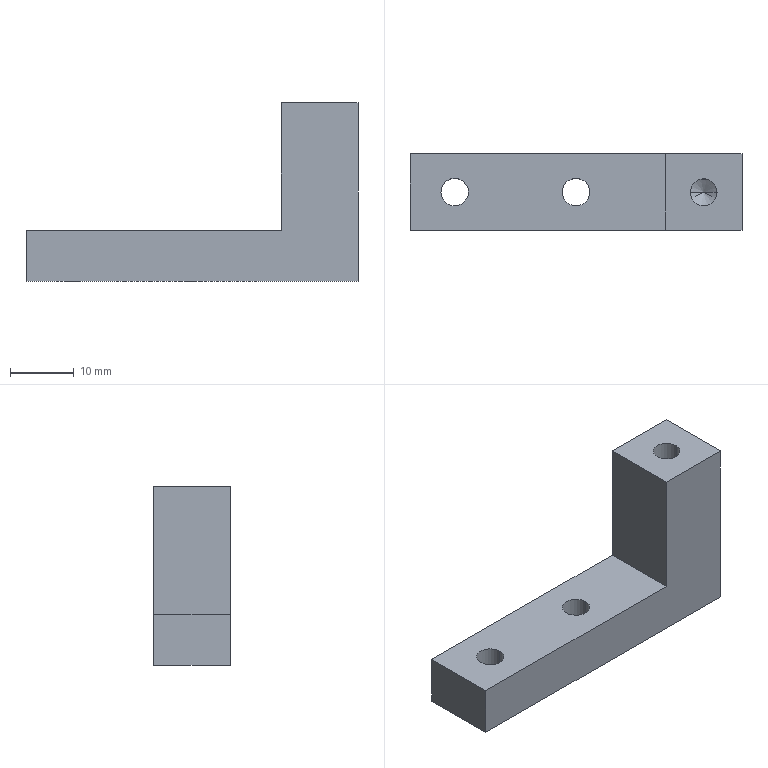Part | STEP file | PN_0008 | 1 solid | 16 faces | box 52 x 12 x 28 mm | volume 7462 mm3 | plane 8 | cylinder 6 | cone 2 | commonest cylinder face diameters 4.3 x4 4.2 x2
STEP:
#1=CARTESIAN_POINT('',(0.,0.,0.));
#2=DIRECTION('',(0.,0.,1.));
#3=DIRECTION('',(1.,0.,0.));
#4=AXIS2_PLACEMENT_3D('',#1,#2,#3);
#5=CARTESIAN_POINT('',(-35.15,6.,0.));
#6=VERTEX_POINT('',#5);
#7=CARTESIAN_POINT('',(-35.15,6.,-8.));
#8=VERTEX_POINT('',#7);
#9=CARTESIAN_POINT('',(-35.15,6.,-8.));
#10=DIRECTION('',(0.,0.,-1.));
#11=VECTOR('',#10,1.);
#12=LINE('',#9,#11);
#13=CARTESIAN_POINT('',(-33.,6.,-8.));
#14=DIRECTION('',(0.,0.,-1.));
#15=DIRECTION('',(-1.,0.,0.));
#16=AXIS2_PLACEMENT_3D('',#13,#14,#15);
#17=CYLINDRICAL_SURFACE('',#16,2.15);
#18=CARTESIAN_POINT('',(6.283,0.));
#19=DIRECTION('',(0.,1.));
#20=VECTOR('',#19,1.);
#21=LINE('',#18,#20);
#22=(GEOMETRIC_REPRESENTATION_CONTEXT(2)PARAMETRIC_REPRESENTATION_CONTEXT()REPRESENTATION_CONTEXT('',''));
#23=DEFINITIONAL_REPRESENTATION('',(#21),#22);
#24=PCURVE('',#17,#23);
#25=CARTESIAN_POINT('',(-33.,6.,-8.));
#26=DIRECTION('',(0.,0.,-1.));
#27=DIRECTION('',(-1.,0.,0.));
#28=AXIS2_PLACEMENT_3D('',#25,#26,#27);
#29=CYLINDRICAL_SURFACE('',#28,2.15);
#30=CARTESIAN_POINT('',(0.,0.));
#31=DIRECTION('',(0.,1.));
#32=VECTOR('',#31,1.);
#33=LINE('',#30,#32);
#34=(GEOMETRIC_REPRESENTATION_CONTEXT(2)PARAMETRIC_REPRESENTATION_CONTEXT()REPRESENTATION_CONTEXT('',''));
#35=DEFINITIONAL_REPRESENTATION('',(#33),#34);
#36=PCURVE('',#29,#35);
#37=SURFACE_CURVE('',#12,(#24,#36),.PCURVE_S1.);
#38=EDGE_CURVE('',#6,#8,#37,.T.);
#39=ORIENTED_EDGE('',*,*,#38,.T.);
#40=CARTESIAN_POINT('',(-30.85,6.,-8.));
#41=VERTEX_POINT('',#40);
#42=CARTESIAN_POINT('',(-33.,6.,-8.));
#43=DIRECTION('',(0.,0.,-1.));
#44=DIRECTION('',(-1.,0.,0.));
#45=AXIS2_PLACEMENT_3D('',#42,#43,#44);
#46=CIRCLE('',#45,2.15);
#47=CARTESIAN_POINT('',(0.,0.));
#48=DIRECTION('',(1.,0.));
#49=VECTOR('',#48,1.);
#50=LINE('',#47,#49);
#51=(GEOMETRIC_REPRESENTATION_CONTEXT(2)PARAMETRIC_REPRESENTATION_CONTEXT()REPRESENTATION_CONTEXT('',''));
#52=DEFINITIONAL_REPRESENTATION('',(#50),#51);
#53=PCURVE('',#17,#52);
#54=CARTESIAN_POINT('',(12.,12.,-8.));
#55=DIRECTION('',(0.,0.,1.));
#56=DIRECTION('',(1.,0.,0.));
#57=AXIS2_PLACEMENT_3D('',#54,#55,#56);
#58=PLANE('',#57);
#59=CARTESIAN_POINT('',(-47.15,-6.));
#60=CARTESIAN_POINT('',(-47.15,-2.276));
#61=CARTESIAN_POINT('',(-43.925,-4.138));
#62=CARTESIAN_POINT('',(-40.7,-6.));
#63=CARTESIAN_POINT('',(-43.925,-7.862));
#64=CARTESIAN_POINT('',(-47.15,-9.724));
#65=CARTESIAN_POINT('',(-47.15,-6.));
#66=(BOUNDED_CURVE()B_SPLINE_CURVE(2,(#59,#60,#61,#62,#63,#64,#65),.UNSPECIFIED.,.T.,.F.)B_SPLINE_CURVE_WITH_KNOTS((1,2,2,2,2,1),(-2.094,0.,2.094,4.189,6.283,8.378),.UNSPECIFIED.)CURVE()GEOMETRIC_REPRESENTATION_ITEM()RATIONAL_B_SPLINE_CURVE((1.,0.5,1.,0.5,1.,0.5,1.))REPRESENTATION_ITEM(''));
#67=(GEOMETRIC_REPRESENTATION_CONTEXT(2)PARAMETRIC_REPRESENTATION_CONTEXT()REPRESENTATION_CONTEXT('',''));
#68=DEFINITIONAL_REPRESENTATION('',(#66),#67);
#69=PCURVE('',#58,#68);
#70=SURFACE_CURVE('',#46,(#53,#69),.PCURVE_S1.);
#71=EDGE_CURVE('',#41,#8,#70,.T.);
#72=ORIENTED_EDGE('',*,*,#71,.F.);
#73=CARTESIAN_POINT('',(-30.85,6.,0.));
#74=VERTEX_POINT('',#73);
#75=CARTESIAN_POINT('',(-30.85,6.,-8.));
#76=DIRECTION('',(0.,0.,-1.));
#77=VECTOR('',#76,1.);
#78=LINE('',#75,#77);
#79=CARTESIAN_POINT('',(3.142,0.));
#80=DIRECTION('',(0.,1.));
#81=VECTOR('',#80,1.);
#82=LINE('',#79,#81);
#83=(GEOMETRIC_REPRESENTATION_CONTEXT(2)PARAMETRIC_REPRESENTATION_CONTEXT()REPRESENTATION_CONTEXT('',''));
#84=DEFINITIONAL_REPRESENTATION('',(#82),#83);
#85=PCURVE('',#17,#84);
#86=CARTESIAN_POINT('',(3.142,0.));
#87=DIRECTION('',(0.,1.));
#88=VECTOR('',#87,1.);
#89=LINE('',#86,#88);
#90=(GEOMETRIC_REPRESENTATION_CONTEXT(2)PARAMETRIC_REPRESENTATION_CONTEXT()REPRESENTATION_CONTEXT('',''));
#91=DEFINITIONAL_REPRESENTATION('',(#89),#90);
#92=PCURVE('',#29,#91);
#93=SURFACE_CURVE('',#78,(#85,#92),.PCURVE_S1.);
#94=EDGE_CURVE('',#74,#41,#93,.T.);
#95=ORIENTED_EDGE('',*,*,#94,.F.);
#96=CARTESIAN_POINT('',(-33.,6.,0.));
#97=DIRECTION('',(0.,0.,-1.));
#98=DIRECTION('',(-1.,0.,0.));
#99=AXIS2_PLACEMENT_3D('',#96,#97,#98);
#100=CIRCLE('',#99,2.15);
#101=CARTESIAN_POINT('',(0.,-8.));
#102=DIRECTION('',(1.,0.));
#103=VECTOR('',#102,1.);
#104=LINE('',#101,#103);
#105=(GEOMETRIC_REPRESENTATION_CONTEXT(2)PARAMETRIC_REPRESENTATION_CONTEXT()REPRESENTATION_CONTEXT('',''));
#106=DEFINITIONAL_REPRESENTATION('',(#104),#105);
#107=PCURVE('',#17,#106);
#108=CARTESIAN_POINT('',(-40.,12.,0.));
#109=DIRECTION('',(0.,0.,-1.));
#110=DIRECTION('',(-1.,0.,0.));
#111=AXIS2_PLACEMENT_3D('',#108,#109,#110);
#112=PLANE('',#111);
#113=CARTESIAN_POINT('',(-7.,-6.));
#114=DIRECTION('',(1.,0.));
#115=AXIS2_PLACEMENT_2D('',#113,#114);
#116=CIRCLE('',#115,2.15);
#117=(GEOMETRIC_REPRESENTATION_CONTEXT(2)PARAMETRIC_REPRESENTATION_CONTEXT()REPRESENTATION_CONTEXT('',''));
#118=DEFINITIONAL_REPRESENTATION('',(#116),#117);
#119=PCURVE('',#112,#118);
#120=SURFACE_CURVE('',#100,(#107,#119),.PCURVE_S1.);
#121=EDGE_CURVE('',#74,#6,#120,.T.);
#122=ORIENTED_EDGE('',*,*,#121,.T.);
#123=EDGE_LOOP('',(#39,#72,#95,#122));
#124=FACE_BOUND('',#123,.F.);
#125=ADVANCED_FACE('',(#124),#17,.F.);
#126=CARTESIAN_POINT('',(-16.15,6.,0.));
#127=VERTEX_POINT('',#126);
#128=CARTESIAN_POINT('',(-16.15,6.,-8.));
#129=VERTEX_POINT('',#128);
#130=CARTESIAN_POINT('',(-16.15,6.,-8.));
#131=DIRECTION('',(0.,0.,-1.));
#132=VECTOR('',#131,1.);
#133=LINE('',#130,#132);
#134=CARTESIAN_POINT('',(-14.,6.,-8.));
#135=DIRECTION('',(0.,0.,-1.));
#136=DIRECTION('',(-1.,0.,0.));
#137=AXIS2_PLACEMENT_3D('',#134,#135,#136);
#138=CYLINDRICAL_SURFACE('',#137,2.15);
#139=CARTESIAN_POINT('',(6.283,0.));
#140=DIRECTION('',(0.,1.));
#141=VECTOR('',#140,1.);
#142=LINE('',#139,#141);
#143=(GEOMETRIC_REPRESENTATION_CONTEXT(2)PARAMETRIC_REPRESENTATION_CONTEXT()REPRESENTATION_CONTEXT('',''));
#144=DEFINITIONAL_REPRESENTATION('',(#142),#143);
#145=PCURVE('',#138,#144);
#146=CARTESIAN_POINT('',(-14.,6.,-8.));
#147=DIRECTION('',(0.,0.,-1.));
#148=DIRECTION('',(-1.,0.,0.));
#149=AXIS2_PLACEMENT_3D('',#146,#147,#148);
#150=CYLINDRICAL_SURFACE('',#149,2.15);
#151=CARTESIAN_POINT('',(0.,0.));
#152=DIRECTION('',(0.,1.));
#153=VECTOR('',#152,1.);
#154=LINE('',#151,#153);
#155=(GEOMETRIC_REPRESENTATION_CONTEXT(2)PARAMETRIC_REPRESENTATION_CONTEXT()REPRESENTATION_CONTEXT('',''));
#156=DEFINITIONAL_REPRESENTATION('',(#154),#155);
#157=PCURVE('',#150,#156);
#158=SURFACE_CURVE('',#133,(#145,#157),.PCURVE_S1.);
#159=EDGE_CURVE('',#127,#129,#158,.T.);
#160=ORIENTED_EDGE('',*,*,#159,.T.);
#161=CARTESIAN_POINT('',(-11.85,6.,-8.));
#162=VERTEX_POINT('',#161);
#163=CARTESIAN_POINT('',(-14.,6.,-8.));
#164=DIRECTION('',(0.,0.,-1.));
#165=DIRECTION('',(-1.,0.,0.));
#166=AXIS2_PLACEMENT_3D('',#163,#164,#165);
#167=CIRCLE('',#166,2.15);
#168=CARTESIAN_POINT('',(0.,0.));
#169=DIRECTION('',(1.,0.));
#170=VECTOR('',#169,1.);
#171=LINE('',#168,#170);
#172=(GEOMETRIC_REPRESENTATION_CONTEXT(2)PARAMETRIC_REPRESENTATION_CONTEXT()REPRESENTATION_CONTEXT('',''));
#173=DEFINITIONAL_REPRESENTATION('',(#171),#172);
#174=PCURVE('',#138,#173);
#175=CARTESIAN_POINT('',(-28.15,-6.));
#176=CARTESIAN_POINT('',(-28.15,-2.276));
#177=CARTESIAN_POINT('',(-24.925,-4.138));
#178=CARTESIAN_POINT('',(-21.7,-6.));
#179=CARTESIAN_POINT('',(-24.925,-7.862));
#180=CARTESIAN_POINT('',(-28.15,-9.724));
#181=CARTESIAN_POINT('',(-28.15,-6.));
#182=(BOUNDED_CURVE()B_SPLINE_CURVE(2,(#175,#176,#177,#178,#179,#180,#181),.UNSPECIFIED.,.T.,.F.)B_SPLINE_CURVE_WITH_KNOTS((1,2,2,2,2,1),(-2.094,0.,2.094,4.189,6.283,8.378),.UNSPECIFIED.)CURVE()GEOMETRIC_REPRESENTATION_ITEM()RATIONAL_B_SPLINE_CURVE((1.,0.5,1.,0.5,1.,0.5,1.))REPRESENTATION_ITEM(''));
#183=(GEOMETRIC_REPRESENTATION_CONTEXT(2)PARAMETRIC_REPRESENTATION_CONTEXT()REPRESENTATION_CONTEXT('',''));
#184=DEFINITIONAL_REPRESENTATION('',(#182),#183);
#185=PCURVE('',#58,#184);
#186=SURFACE_CURVE('',#167,(#174,#185),.PCURVE_S1.);
#187=EDGE_CURVE('',#162,#129,#186,.T.);
#188=ORIENTED_EDGE('',*,*,#187,.F.);
#189=CARTESIAN_POINT('',(-11.85,6.,0.));
#190=VERTEX_POINT('',#189);
#191=CARTESIAN_POINT('',(-11.85,6.,-8.));
#192=DIRECTION('',(0.,0.,-1.));
#193=VECTOR('',#192,1.);
#194=LINE('',#191,#193);
#195=CARTESIAN_POINT('',(3.142,0.));
#196=DIRECTION('',(0.,1.));
#197=VECTOR('',#196,1.);
#198=LINE('',#195,#197);
#199=(GEOMETRIC_REPRESENTATION_CONTEXT(2)PARAMETRIC_REPRESENTATION_CONTEXT()REPRESENTATION_CONTEXT('',''));
#200=DEFINITIONAL_REPRESENTATION('',(#198),#199);
#201=PCURVE('',#138,#200);
#202=CARTESIAN_POINT('',(3.142,0.));
#203=DIRECTION('',(0.,1.));
#204=VECTOR('',#203,1.);
#205=LINE('',#202,#204);
#206=(GEOMETRIC_REPRESENTATION_CONTEXT(2)PARAMETRIC_REPRESENTATION_CONTEXT()REPRESENTATION_CONTEXT('',''));
#207=DEFINITIONAL_REPRESENTATION('',(#205),#206);
#208=PCURVE('',#150,#207);
#209=SURFACE_CURVE('',#194,(#201,#208),.PCURVE_S1.);
#210=EDGE_CURVE('',#190,#162,#209,.T.);
#211=ORIENTED_EDGE('',*,*,#210,.F.);
#212=CARTESIAN_POINT('',(-14.,6.,0.));
#213=DIRECTION('',(0.,0.,-1.));
#214=DIRECTION('',(-1.,0.,0.));
#215=AXIS2_PLACEMENT_3D('',#212,#213,#214);
#216=CIRCLE('',#215,2.15);
#217=CARTESIAN_POINT('',(0.,-8.));
#218=DIRECTION('',(1.,0.));
#219=VECTOR('',#218,1.);
#220=LINE('',#217,#219);
#221=(GEOMETRIC_REPRESENTATION_CONTEXT(2)PARAMETRIC_REPRESENTATION_CONTEXT()REPRESENTATION_CONTEXT('',''));
#222=DEFINITIONAL_REPRESENTATION('',(#220),#221);
#223=PCURVE('',#138,#222);
#224=CARTESIAN_POINT('',(-26.,-6.));
#225=DIRECTION('',(1.,0.));
#226=AXIS2_PLACEMENT_2D('',#224,#225);
#227=CIRCLE('',#226,2.15);
#228=(GEOMETRIC_REPRESENTATION_CONTEXT(2)PARAMETRIC_REPRESENTATION_CONTEXT()REPRESENTATION_CONTEXT('',''));
#229=DEFINITIONAL_REPRESENTATION('',(#227),#228);
#230=PCURVE('',#112,#229);
#231=SURFACE_CURVE('',#216,(#223,#230),.PCURVE_S1.);
#232=EDGE_CURVE('',#190,#127,#231,.T.);
#233=ORIENTED_EDGE('',*,*,#232,.T.);
#234=EDGE_LOOP('',(#160,#188,#211,#233));
#235=FACE_BOUND('',#234,.F.);
#236=ADVANCED_FACE('',(#235),#138,.F.);
#237=CARTESIAN_POINT('',(8.1,5.929,7.6));
#238=VERTEX_POINT('',#237);
#239=CARTESIAN_POINT('',(8.1,5.929,20.));
#240=VERTEX_POINT('',#239);
#241=CARTESIAN_POINT('',(8.1,5.929,20.));
#242=DIRECTION('',(0.,0.,1.));
#243=VECTOR('',#242,1.);
#244=LINE('',#241,#243);
#245=CARTESIAN_POINT('',(6.,5.929,20.));
#246=DIRECTION('',(0.,0.,1.));
#247=DIRECTION('',(1.,0.,0.));
#248=AXIS2_PLACEMENT_3D('',#245,#246,#247);
#249=CYLINDRICAL_SURFACE('',#248,2.1);
#250=CARTESIAN_POINT('',(6.283,0.));
#251=DIRECTION('',(0.,1.));
#252=VECTOR('',#251,1.);
#253=LINE('',#250,#252);
#254=(GEOMETRIC_REPRESENTATION_CONTEXT(2)PARAMETRIC_REPRESENTATION_CONTEXT()REPRESENTATION_CONTEXT('',''));
#255=DEFINITIONAL_REPRESENTATION('',(#253),#254);
#256=PCURVE('',#249,#255);
#257=CARTESIAN_POINT('',(6.,5.929,20.));
#258=DIRECTION('',(0.,0.,1.));
#259=DIRECTION('',(1.,0.,0.));
#260=AXIS2_PLACEMENT_3D('',#257,#258,#259);
#261=CYLINDRICAL_SURFACE('',#260,2.1);
#262=CARTESIAN_POINT('',(0.,0.));
#263=DIRECTION('',(0.,1.));
#264=VECTOR('',#263,1.);
#265=LINE('',#262,#264);
#266=(GEOMETRIC_REPRESENTATION_CONTEXT(2)PARAMETRIC_REPRESENTATION_CONTEXT()REPRESENTATION_CONTEXT('',''));
#267=DEFINITIONAL_REPRESENTATION('',(#265),#266);
#268=PCURVE('',#261,#267);
#269=SURFACE_CURVE('',#244,(#256,#268),.PCURVE_S1.);
#270=EDGE_CURVE('',#238,#240,#269,.T.);
#271=ORIENTED_EDGE('',*,*,#270,.T.);
#272=CARTESIAN_POINT('',(3.9,5.929,20.));
#273=VERTEX_POINT('',#272);
#274=CARTESIAN_POINT('',(6.,5.929,20.));
#275=DIRECTION('',(0.,0.,1.));
#276=DIRECTION('',(1.,0.,0.));
#277=AXIS2_PLACEMENT_3D('',#274,#275,#276);
#278=CIRCLE('',#277,2.1);
#279=CARTESIAN_POINT('',(0.,0.));
#280=DIRECTION('',(1.,0.));
#281=VECTOR('',#280,1.);
#282=LINE('',#279,#281);
#283=(GEOMETRIC_REPRESENTATION_CONTEXT(2)PARAMETRIC_REPRESENTATION_CONTEXT()REPRESENTATION_CONTEXT('',''));
#284=DEFINITIONAL_REPRESENTATION('',(#282),#283);
#285=PCURVE('',#249,#284);
#286=CARTESIAN_POINT('',(0.,12.,20.));
#287=DIRECTION('',(0.,0.,-1.));
#288=DIRECTION('',(-1.,0.,0.));
#289=AXIS2_PLACEMENT_3D('',#286,#287,#288);
#290=PLANE('',#289);
#291=CARTESIAN_POINT('',(-8.1,-6.071));
#292=CARTESIAN_POINT('',(-8.1,-2.433));
#293=CARTESIAN_POINT('',(-4.95,-4.252));
#294=CARTESIAN_POINT('',(-1.8,-6.071));
#295=CARTESIAN_POINT('',(-4.95,-7.889));
#296=CARTESIAN_POINT('',(-8.1,-9.708));
#297=CARTESIAN_POINT('',(-8.1,-6.071));
#298=(BOUNDED_CURVE()B_SPLINE_CURVE(2,(#291,#292,#293,#294,#295,#296,#297),.UNSPECIFIED.,.T.,.F.)B_SPLINE_CURVE_WITH_KNOTS((1,2,2,2,2,1),(-2.094,0.,2.094,4.189,6.283,8.378),.UNSPECIFIED.)CURVE()GEOMETRIC_REPRESENTATION_ITEM()RATIONAL_B_SPLINE_CURVE((1.,0.5,1.,0.5,1.,0.5,1.))REPRESENTATION_ITEM(''));
#299=(GEOMETRIC_REPRESENTATION_CONTEXT(2)PARAMETRIC_REPRESENTATION_CONTEXT()REPRESENTATION_CONTEXT('',''));
#300=DEFINITIONAL_REPRESENTATION('',(#298),#299);
#301=PCURVE('',#290,#300);
#302=SURFACE_CURVE('',#278,(#285,#301),.PCURVE_S1.);
#303=EDGE_CURVE('',#273,#240,#302,.T.);
#304=ORIENTED_EDGE('',*,*,#303,.F.);
#305=CARTESIAN_POINT('',(3.9,5.929,7.6));
#306=VERTEX_POINT('',#305);
#307=CARTESIAN_POINT('',(3.9,5.929,20.));
#308=DIRECTION('',(0.,0.,1.));
#309=VECTOR('',#308,1.);
#310=LINE('',#307,#309);
#311=CARTESIAN_POINT('',(3.142,0.));
#312=DIRECTION('',(0.,1.));
#313=VECTOR('',#312,1.);
#314=LINE('',#311,#313);
#315=(GEOMETRIC_REPRESENTATION_CONTEXT(2)PARAMETRIC_REPRESENTATION_CONTEXT()REPRESENTATION_CONTEXT('',''));
#316=DEFINITIONAL_REPRESENTATION('',(#314),#315);
#317=PCURVE('',#249,#316);
#318=CARTESIAN_POINT('',(3.142,0.));
#319=DIRECTION('',(0.,1.));
#320=VECTOR('',#319,1.);
#321=LINE('',#318,#320);
#322=(GEOMETRIC_REPRESENTATION_CONTEXT(2)PARAMETRIC_REPRESENTATION_CONTEXT()REPRESENTATION_CONTEXT('',''));
#323=DEFINITIONAL_REPRESENTATION('',(#321),#322);
#324=PCURVE('',#261,#323);
#325=SURFACE_CURVE('',#310,(#317,#324),.PCURVE_S1.);
#326=EDGE_CURVE('',#306,#273,#325,.T.);
#327=ORIENTED_EDGE('',*,*,#326,.F.);
#328=CARTESIAN_POINT('',(6.,5.929,7.6));
#329=DIRECTION('',(0.,0.,1.));
#330=DIRECTION('',(1.,0.,0.));
#331=AXIS2_PLACEMENT_3D('',#328,#329,#330);
#332=CIRCLE('',#331,2.1);
#333=CARTESIAN_POINT('',(0.,-12.4));
#334=DIRECTION('',(1.,0.));
#335=VECTOR('',#334,1.);
#336=LINE('',#333,#335);
#337=(GEOMETRIC_REPRESENTATION_CONTEXT(2)PARAMETRIC_REPRESENTATION_CONTEXT()REPRESENTATION_CONTEXT('',''));
#338=DEFINITIONAL_REPRESENTATION('',(#336),#337);
#339=PCURVE('',#249,#338);
#340=CARTESIAN_POINT('',(6.,5.929,7.6));
#341=DIRECTION('',(0.,0.,1.));
#342=DIRECTION('',(1.,0.,0.));
#343=AXIS2_PLACEMENT_3D('',#340,#341,#342);
#344=CONICAL_SURFACE('',#343,2.1,1.03);
#345=CARTESIAN_POINT('',(0.,0.));
#346=DIRECTION('',(1.,0.));
#347=VECTOR('',#346,1.);
#348=LINE('',#345,#347);
#349=(GEOMETRIC_REPRESENTATION_CONTEXT(2)PARAMETRIC_REPRESENTATION_CONTEXT()REPRESENTATION_CONTEXT('',''));
#350=DEFINITIONAL_REPRESENTATION('',(#348),#349);
#351=PCURVE('',#344,#350);
#352=SURFACE_CURVE('',#332,(#339,#351),.PCURVE_S1.);
#353=EDGE_CURVE('',#306,#238,#352,.T.);
#354=ORIENTED_EDGE('',*,*,#353,.T.);
#355=EDGE_LOOP('',(#271,#304,#327,#354));
#356=FACE_BOUND('',#355,.F.);
#357=ADVANCED_FACE('',(#356),#249,.F.);
#358=ORIENTED_EDGE('',*,*,#353,.F.);
#359=CARTESIAN_POINT('',(6.,5.929,6.338));
#360=VERTEX_POINT('',#359);
#361=CARTESIAN_POINT('',(3.9,5.929,7.6));
#362=DIRECTION('',(-0.8572,0.,0.515));
#363=VECTOR('',#362,1.);
#364=LINE('',#361,#363);
#365=CARTESIAN_POINT('',(3.142,0.));
#366=DIRECTION('',(0.,1.));
#367=VECTOR('',#366,1.);
#368=LINE('',#365,#367);
#369=(GEOMETRIC_REPRESENTATION_CONTEXT(2)PARAMETRIC_REPRESENTATION_CONTEXT()REPRESENTATION_CONTEXT('',''));
#370=DEFINITIONAL_REPRESENTATION('',(#368),#369);
#371=PCURVE('',#344,#370);
#372=CARTESIAN_POINT('',(6.,5.929,7.6));
#373=DIRECTION('',(0.,0.,1.));
#374=DIRECTION('',(1.,0.,0.));
#375=AXIS2_PLACEMENT_3D('',#372,#373,#374);
#376=CONICAL_SURFACE('',#375,2.1,1.03);
#377=CARTESIAN_POINT('',(3.142,0.));
#378=DIRECTION('',(0.,1.));
#379=VECTOR('',#378,1.);
#380=LINE('',#377,#379);
#381=(GEOMETRIC_REPRESENTATION_CONTEXT(2)PARAMETRIC_REPRESENTATION_CONTEXT()REPRESENTATION_CONTEXT('',''));
#382=DEFINITIONAL_REPRESENTATION('',(#380),#381);
#383=PCURVE('',#376,#382);
#384=SURFACE_CURVE('',#364,(#371,#383),.PCURVE_S1.);
#385=EDGE_CURVE('',#360,#306,#384,.T.);
#386=ORIENTED_EDGE('',*,*,#385,.F.);
#387=CARTESIAN_POINT('',(8.1,5.929,7.6));
#388=DIRECTION('',(0.8572,0.,0.515));
#389=VECTOR('',#388,1.);
#390=LINE('',#387,#389);
#391=CARTESIAN_POINT('',(6.283,0.));
#392=DIRECTION('',(0.,1.));
#393=VECTOR('',#392,1.);
#394=LINE('',#391,#393);
#395=(GEOMETRIC_REPRESENTATION_CONTEXT(2)PARAMETRIC_REPRESENTATION_CONTEXT()REPRESENTATION_CONTEXT('',''));
#396=DEFINITIONAL_REPRESENTATION('',(#394),#395);
#397=PCURVE('',#344,#396);
#398=CARTESIAN_POINT('',(0.,0.));
#399=DIRECTION('',(0.,1.));
#400=VECTOR('',#399,1.);
#401=LINE('',#398,#400);
#402=(GEOMETRIC_REPRESENTATION_CONTEXT(2)PARAMETRIC_REPRESENTATION_CONTEXT()REPRESENTATION_CONTEXT('',''));
#403=DEFINITIONAL_REPRESENTATION('',(#401),#402);
#404=PCURVE('',#376,#403);
#405=SURFACE_CURVE('',#390,(#397,#404),.PCURVE_S1.);
#406=EDGE_CURVE('',#360,#238,#405,.T.);
#407=ORIENTED_EDGE('',*,*,#406,.T.);
#408=EDGE_LOOP('',(#358,#386,#407));
#409=FACE_BOUND('',#408,.F.);
#410=ADVANCED_FACE('',(#409),#344,.F.);
#411=CARTESIAN_POINT('',(-40.,0.,-8.));
#412=VERTEX_POINT('',#411);
#413=CARTESIAN_POINT('',(-40.,0.,0.));
#414=VERTEX_POINT('',#413);
#415=CARTESIAN_POINT('',(-40.,0.,-8.));
#416=DIRECTION('',(0.,0.,1.));
#417=VECTOR('',#416,1.);
#418=LINE('',#415,#417);
#419=CARTESIAN_POINT('',(-40.,12.,-8.));
#420=DIRECTION('',(1.,0.,0.));
#421=DIRECTION('',(0.,0.,-1.));
#422=AXIS2_PLACEMENT_3D('',#419,#420,#421);
#423=PLANE('',#422);
#424=CARTESIAN_POINT('',(0.,-12.));
#425=DIRECTION('',(-1.,0.));
#426=VECTOR('',#425,1.);
#427=LINE('',#424,#426);
#428=(GEOMETRIC_REPRESENTATION_CONTEXT(2)PARAMETRIC_REPRESENTATION_CONTEXT()REPRESENTATION_CONTEXT('',''));
#429=DEFINITIONAL_REPRESENTATION('',(#427),#428);
#430=PCURVE('',#423,#429);
#431=CARTESIAN_POINT('',(0.,0.,0.));
#432=DIRECTION('',(0.,1.,0.));
#433=DIRECTION('',(0.,0.,1.));
#434=AXIS2_PLACEMENT_3D('',#431,#432,#433);
#435=PLANE('',#434);
#436=CARTESIAN_POINT('',(-8.,-40.));
#437=DIRECTION('',(1.,0.));
#438=VECTOR('',#437,1.);
#439=LINE('',#436,#438);
#440=(GEOMETRIC_REPRESENTATION_CONTEXT(2)PARAMETRIC_REPRESENTATION_CONTEXT()REPRESENTATION_CONTEXT('',''));
#441=DEFINITIONAL_REPRESENTATION('',(#439),#440);
#442=PCURVE('',#435,#441);
#443=SURFACE_CURVE('',#418,(#430,#442),.PCURVE_S1.);
#444=EDGE_CURVE('',#412,#414,#443,.T.);
#445=ORIENTED_EDGE('',*,*,#444,.T.);
#446=CARTESIAN_POINT('',(-40.,12.,0.));
#447=VERTEX_POINT('',#446);
#448=CARTESIAN_POINT('',(-40.,12.,0.));
#449=DIRECTION('',(0.,-1.,0.));
#450=VECTOR('',#449,1.);
#451=LINE('',#448,#450);
#452=CARTESIAN_POINT('',(-8.,0.));
#453=DIRECTION('',(0.,-1.));
#454=VECTOR('',#453,1.);
#455=LINE('',#452,#454);
#456=(GEOMETRIC_REPRESENTATION_CONTEXT(2)PARAMETRIC_REPRESENTATION_CONTEXT()REPRESENTATION_CONTEXT('',''));
#457=DEFINITIONAL_REPRESENTATION('',(#455),#456);
#458=PCURVE('',#423,#457);
#459=CARTESIAN_POINT('',(0.,0.));
#460=DIRECTION('',(0.,-1.));
#461=VECTOR('',#460,1.);
#462=LINE('',#459,#461);
#463=(GEOMETRIC_REPRESENTATION_CONTEXT(2)PARAMETRIC_REPRESENTATION_CONTEXT()REPRESENTATION_CONTEXT('',''));
#464=DEFINITIONAL_REPRESENTATION('',(#462),#463);
#465=PCURVE('',#112,#464);
#466=SURFACE_CURVE('',#451,(#458,#465),.PCURVE_S1.);
#467=EDGE_CURVE('',#447,#414,#466,.T.);
#468=ORIENTED_EDGE('',*,*,#467,.F.);
#469=CARTESIAN_POINT('',(-40.,12.,-8.));
#470=VERTEX_POINT('',#469);
#471=CARTESIAN_POINT('',(-40.,12.,-8.));
#472=DIRECTION('',(0.,0.,1.));
#473=VECTOR('',#472,1.);
#474=LINE('',#471,#473);
#475=CARTESIAN_POINT('',(0.,0.));
#476=DIRECTION('',(-1.,0.));
#477=VECTOR('',#476,1.);
#478=LINE('',#475,#477);
#479=(GEOMETRIC_REPRESENTATION_CONTEXT(2)PARAMETRIC_REPRESENTATION_CONTEXT()REPRESENTATION_CONTEXT('',''));
#480=DEFINITIONAL_REPRESENTATION('',(#478),#479);
#481=PCURVE('',#423,#480);
#482=CARTESIAN_POINT('',(0.,12.,0.));
#483=DIRECTION('',(0.,1.,0.));
#484=DIRECTION('',(0.,0.,1.));
#485=AXIS2_PLACEMENT_3D('',#482,#483,#484);
#486=PLANE('',#485);
#487=CARTESIAN_POINT('',(-8.,-40.));
#488=DIRECTION('',(1.,0.));
#489=VECTOR('',#488,1.);
#490=LINE('',#487,#489);
#491=(GEOMETRIC_REPRESENTATION_CONTEXT(2)PARAMETRIC_REPRESENTATION_CONTEXT()REPRESENTATION_CONTEXT('',''));
#492=DEFINITIONAL_REPRESENTATION('',(#490),#491);
#493=PCURVE('',#486,#492);
#494=SURFACE_CURVE('',#474,(#481,#493),.PCURVE_S1.);
#495=EDGE_CURVE('',#470,#447,#494,.T.);
#496=ORIENTED_EDGE('',*,*,#495,.F.);
#497=CARTESIAN_POINT('',(-40.,12.,-8.));
#498=DIRECTION('',(0.,-1.,0.));
#499=VECTOR('',#498,1.);
#500=LINE('',#497,#499);
#501=CARTESIAN_POINT('',(0.,0.));
#502=DIRECTION('',(0.,-1.));
#503=VECTOR('',#502,1.);
#504=LINE('',#501,#503);
#505=(GEOMETRIC_REPRESENTATION_CONTEXT(2)PARAMETRIC_REPRESENTATION_CONTEXT()REPRESENTATION_CONTEXT('',''));
#506=DEFINITIONAL_REPRESENTATION('',(#504),#505);
#507=PCURVE('',#423,#506);
#508=CARTESIAN_POINT('',(-52.,0.));
#509=DIRECTION('',(0.,-1.));
#510=VECTOR('',#509,1.);
#511=LINE('',#508,#510);
#512=(GEOMETRIC_REPRESENTATION_CONTEXT(2)PARAMETRIC_REPRESENTATION_CONTEXT()REPRESENTATION_CONTEXT('',''));
#513=DEFINITIONAL_REPRESENTATION('',(#511),#512);
#514=PCURVE('',#58,#513);
#515=SURFACE_CURVE('',#500,(#507,#514),.PCURVE_S1.);
#516=EDGE_CURVE('',#470,#412,#515,.T.);
#517=ORIENTED_EDGE('',*,*,#516,.T.);
#518=EDGE_LOOP('',(#445,#468,#496,#517));
#519=FACE_BOUND('',#518,.T.);
#520=ADVANCED_FACE('',(#519),#423,.F.);
#521=CARTESIAN_POINT('',(-33.,6.,0.));
#522=DIRECTION('',(0.,0.,-1.));
#523=DIRECTION('',(-1.,0.,0.));
#524=AXIS2_PLACEMENT_3D('',#521,#522,#523);
#525=CIRCLE('',#524,2.15);
#526=CARTESIAN_POINT('',(-7.,-6.));
#527=DIRECTION('',(1.,0.));
#528=AXIS2_PLACEMENT_2D('',#526,#527);
#529=CIRCLE('',#528,2.15);
#530=(GEOMETRIC_REPRESENTATION_CONTEXT(2)PARAMETRIC_REPRESENTATION_CONTEXT()REPRESENTATION_CONTEXT('',''));
#531=DEFINITIONAL_REPRESENTATION('',(#529),#530);
#532=PCURVE('',#112,#531);
#533=CARTESIAN_POINT('',(0.,-8.));
#534=DIRECTION('',(1.,0.));
#535=VECTOR('',#534,1.);
#536=LINE('',#533,#535);
#537=(GEOMETRIC_REPRESENTATION_CONTEXT(2)PARAMETRIC_REPRESENTATION_CONTEXT()REPRESENTATION_CONTEXT('',''));
#538=DEFINITIONAL_REPRESENTATION('',(#536),#537);
#539=PCURVE('',#29,#538);
#540=SURFACE_CURVE('',#525,(#532,#539),.PCURVE_S1.);
#541=EDGE_CURVE('',#6,#74,#540,.T.);
#542=ORIENTED_EDGE('',*,*,#541,.T.);
#543=ORIENTED_EDGE('',*,*,#121,.T.);
#544=EDGE_LOOP('',(#542,#543));
#545=FACE_BOUND('',#544,.T.);
#546=CARTESIAN_POINT('',(-14.,6.,0.));
#547=DIRECTION('',(0.,0.,-1.));
#548=DIRECTION('',(-1.,0.,0.));
#549=AXIS2_PLACEMENT_3D('',#546,#547,#548);
#550=CIRCLE('',#549,2.15);
#551=CARTESIAN_POINT('',(-26.,-6.));
#552=DIRECTION('',(1.,0.));
#553=AXIS2_PLACEMENT_2D('',#551,#552);
#554=CIRCLE('',#553,2.15);
#555=(GEOMETRIC_REPRESENTATION_CONTEXT(2)PARAMETRIC_REPRESENTATION_CONTEXT()REPRESENTATION_CONTEXT('',''));
#556=DEFINITIONAL_REPRESENTATION('',(#554),#555);
#557=PCURVE('',#112,#556);
#558=CARTESIAN_POINT('',(0.,-8.));
#559=DIRECTION('',(1.,0.));
#560=VECTOR('',#559,1.);
#561=LINE('',#558,#560);
#562=(GEOMETRIC_REPRESENTATION_CONTEXT(2)PARAMETRIC_REPRESENTATION_CONTEXT()REPRESENTATION_CONTEXT('',''));
#563=DEFINITIONAL_REPRESENTATION('',(#561),#562);
#564=PCURVE('',#150,#563);
#565=SURFACE_CURVE('',#550,(#557,#564),.PCURVE_S1.);
#566=EDGE_CURVE('',#127,#190,#565,.T.);
#567=ORIENTED_EDGE('',*,*,#566,.T.);
#568=ORIENTED_EDGE('',*,*,#232,.T.);
#569=EDGE_LOOP('',(#567,#568));
#570=FACE_BOUND('',#569,.T.);
#571=CARTESIAN_POINT('',(0.,0.,0.));
#572=VERTEX_POINT('',#571);
#573=CARTESIAN_POINT('',(-40.,0.,0.));
#574=DIRECTION('',(1.,0.,0.));
#575=VECTOR('',#574,1.);
#576=LINE('',#573,#575);
#577=CARTESIAN_POINT('',(0.,-12.));
#578=DIRECTION('',(-1.,0.));
#579=VECTOR('',#578,1.);
#580=LINE('',#577,#579);
#581=(GEOMETRIC_REPRESENTATION_CONTEXT(2)PARAMETRIC_REPRESENTATION_CONTEXT()REPRESENTATION_CONTEXT('',''));
#582=DEFINITIONAL_REPRESENTATION('',(#580),#581);
#583=PCURVE('',#112,#582);
#584=CARTESIAN_POINT('',(0.,-40.));
#585=DIRECTION('',(0.,1.));
#586=VECTOR('',#585,1.);
#587=LINE('',#584,#586);
#588=(GEOMETRIC_REPRESENTATION_CONTEXT(2)PARAMETRIC_REPRESENTATION_CONTEXT()REPRESENTATION_CONTEXT('',''));
#589=DEFINITIONAL_REPRESENTATION('',(#587),#588);
#590=PCURVE('',#435,#589);
#591=SURFACE_CURVE('',#576,(#583,#590),.PCURVE_S1.);
#592=EDGE_CURVE('',#414,#572,#591,.T.);
#593=ORIENTED_EDGE('',*,*,#592,.T.);
#594=CARTESIAN_POINT('',(0.,12.,0.));
#595=VERTEX_POINT('',#594);
#596=CARTESIAN_POINT('',(0.,12.,0.));
#597=DIRECTION('',(0.,-1.,0.));
#598=VECTOR('',#597,1.);
#599=LINE('',#596,#598);
#600=CARTESIAN_POINT('',(-40.,0.));
#601=DIRECTION('',(0.,-1.));
#602=VECTOR('',#601,1.);
#603=LINE('',#600,#602);
#604=(GEOMETRIC_REPRESENTATION_CONTEXT(2)PARAMETRIC_REPRESENTATION_CONTEXT()REPRESENTATION_CONTEXT('',''));
#605=DEFINITIONAL_REPRESENTATION('',(#603),#604);
#606=PCURVE('',#112,#605);
#607=CARTESIAN_POINT('',(0.,12.,0.));
#608=DIRECTION('',(1.,0.,0.));
#609=DIRECTION('',(0.,0.,-1.));
#610=AXIS2_PLACEMENT_3D('',#607,#608,#609);
#611=PLANE('',#610);
#612=CARTESIAN_POINT('',(0.,0.));
#613=DIRECTION('',(0.,-1.));
#614=VECTOR('',#613,1.);
#615=LINE('',#612,#614);
#616=(GEOMETRIC_REPRESENTATION_CONTEXT(2)PARAMETRIC_REPRESENTATION_CONTEXT()REPRESENTATION_CONTEXT('',''));
#617=DEFINITIONAL_REPRESENTATION('',(#615),#616);
#618=PCURVE('',#611,#617);
#619=SURFACE_CURVE('',#599,(#606,#618),.PCURVE_S1.);
#620=EDGE_CURVE('',#595,#572,#619,.T.);
#621=ORIENTED_EDGE('',*,*,#620,.F.);
#622=CARTESIAN_POINT('',(-40.,12.,0.));
#623=DIRECTION('',(1.,0.,0.));
#624=VECTOR('',#623,1.);
#625=LINE('',#622,#624);
#626=CARTESIAN_POINT('',(0.,0.));
#627=DIRECTION('',(-1.,0.));
#628=VECTOR('',#627,1.);
#629=LINE('',#626,#628);
#630=(GEOMETRIC_REPRESENTATION_CONTEXT(2)PARAMETRIC_REPRESENTATION_CONTEXT()REPRESENTATION_CONTEXT('',''));
#631=DEFINITIONAL_REPRESENTATION('',(#629),#630);
#632=PCURVE('',#112,#631);
#633=CARTESIAN_POINT('',(0.,-40.));
#634=DIRECTION('',(0.,1.));
#635=VECTOR('',#634,1.);
#636=LINE('',#633,#635);
#637=(GEOMETRIC_REPRESENTATION_CONTEXT(2)PARAMETRIC_REPRESENTATION_CONTEXT()REPRESENTATION_CONTEXT('',''));
#638=DEFINITIONAL_REPRESENTATION('',(#636),#637);
#639=PCURVE('',#486,#638);
#640=SURFACE_CURVE('',#625,(#632,#639),.PCURVE_S1.);
#641=EDGE_CURVE('',#447,#595,#640,.T.);
#642=ORIENTED_EDGE('',*,*,#641,.F.);
#643=ORIENTED_EDGE('',*,*,#467,.T.);
#644=EDGE_LOOP('',(#593,#621,#642,#643));
#645=FACE_BOUND('',#644,.T.);
#646=ADVANCED_FACE('',(#545,#570,#645),#112,.F.);
#647=CARTESIAN_POINT('',(0.,0.,20.));
#648=VERTEX_POINT('',#647);
#649=CARTESIAN_POINT('',(0.,0.,0.));
#650=DIRECTION('',(0.,0.,1.));
#651=VECTOR('',#650,1.);
#652=LINE('',#649,#651);
#653=CARTESIAN_POINT('',(0.,-12.));
#654=DIRECTION('',(-1.,0.));
#655=VECTOR('',#654,1.);
#656=LINE('',#653,#655);
#657=(GEOMETRIC_REPRESENTATION_CONTEXT(2)PARAMETRIC_REPRESENTATION_CONTEXT()REPRESENTATION_CONTEXT('',''));
#658=DEFINITIONAL_REPRESENTATION('',(#656),#657);
#659=PCURVE('',#611,#658);
#660=CARTESIAN_POINT('',(0.,0.));
#661=DIRECTION('',(1.,0.));
#662=VECTOR('',#661,1.);
#663=LINE('',#660,#662);
#664=(GEOMETRIC_REPRESENTATION_CONTEXT(2)PARAMETRIC_REPRESENTATION_CONTEXT()REPRESENTATION_CONTEXT('',''));
#665=DEFINITIONAL_REPRESENTATION('',(#663),#664);
#666=PCURVE('',#435,#665);
#667=SURFACE_CURVE('',#652,(#659,#666),.PCURVE_S1.);
#668=EDGE_CURVE('',#572,#648,#667,.T.);
#669=ORIENTED_EDGE('',*,*,#668,.T.);
#670=CARTESIAN_POINT('',(0.,12.,20.));
#671=VERTEX_POINT('',#670);
#672=CARTESIAN_POINT('',(0.,12.,20.));
#673=DIRECTION('',(0.,-1.,0.));
#674=VECTOR('',#673,1.);
#675=LINE('',#672,#674);
#676=CARTESIAN_POINT('',(-20.,0.));
#677=DIRECTION('',(0.,-1.));
#678=VECTOR('',#677,1.);
#679=LINE('',#676,#678);
#680=(GEOMETRIC_REPRESENTATION_CONTEXT(2)PARAMETRIC_REPRESENTATION_CONTEXT()REPRESENTATION_CONTEXT('',''));
#681=DEFINITIONAL_REPRESENTATION('',(#679),#680);
#682=PCURVE('',#611,#681);
#683=CARTESIAN_POINT('',(0.,0.));
#684=DIRECTION('',(0.,-1.));
#685=VECTOR('',#684,1.);
#686=LINE('',#683,#685);
#687=(GEOMETRIC_REPRESENTATION_CONTEXT(2)PARAMETRIC_REPRESENTATION_CONTEXT()REPRESENTATION_CONTEXT('',''));
#688=DEFINITIONAL_REPRESENTATION('',(#686),#687);
#689=PCURVE('',#290,#688);
#690=SURFACE_CURVE('',#675,(#682,#689),.PCURVE_S1.);
#691=EDGE_CURVE('',#671,#648,#690,.T.);
#692=ORIENTED_EDGE('',*,*,#691,.F.);
#693=CARTESIAN_POINT('',(0.,12.,0.));
#694=DIRECTION('',(0.,0.,1.));
#695=VECTOR('',#694,1.);
#696=LINE('',#693,#695);
#697=CARTESIAN_POINT('',(0.,0.));
#698=DIRECTION('',(-1.,0.));
#699=VECTOR('',#698,1.);
#700=LINE('',#697,#699);
#701=(GEOMETRIC_REPRESENTATION_CONTEXT(2)PARAMETRIC_REPRESENTATION_CONTEXT()REPRESENTATION_CONTEXT('',''));
#702=DEFINITIONAL_REPRESENTATION('',(#700),#701);
#703=PCURVE('',#611,#702);
#704=CARTESIAN_POINT('',(0.,0.));
#705=DIRECTION('',(1.,0.));
#706=VECTOR('',#705,1.);
#707=LINE('',#704,#706);
#708=(GEOMETRIC_REPRESENTATION_CONTEXT(2)PARAMETRIC_REPRESENTATION_CONTEXT()REPRESENTATION_CONTEXT('',''));
#709=DEFINITIONAL_REPRESENTATION('',(#707),#708);
#710=PCURVE('',#486,#709);
#711=SURFACE_CURVE('',#696,(#703,#710),.PCURVE_S1.);
#712=EDGE_CURVE('',#595,#671,#711,.T.);
#713=ORIENTED_EDGE('',*,*,#712,.F.);
#714=ORIENTED_EDGE('',*,*,#620,.T.);
#715=EDGE_LOOP('',(#669,#692,#713,#714));
#716=FACE_BOUND('',#715,.T.);
#717=ADVANCED_FACE('',(#716),#611,.F.);
#718=CARTESIAN_POINT('',(6.,5.929,20.));
#719=DIRECTION('',(0.,0.,1.));
#720=DIRECTION('',(1.,0.,0.));
#721=AXIS2_PLACEMENT_3D('',#718,#719,#720);
#722=CIRCLE('',#721,2.1);
#723=CARTESIAN_POINT('',(-8.1,-6.071));
#724=CARTESIAN_POINT('',(-8.1,-2.433));
#725=CARTESIAN_POINT('',(-4.95,-4.252));
#726=CARTESIAN_POINT('',(-1.8,-6.071));
#727=CARTESIAN_POINT('',(-4.95,-7.889));
#728=CARTESIAN_POINT('',(-8.1,-9.708));
#729=CARTESIAN_POINT('',(-8.1,-6.071));
#730=(BOUNDED_CURVE()B_SPLINE_CURVE(2,(#723,#724,#725,#726,#727,#728,#729),.UNSPECIFIED.,.T.,.F.)B_SPLINE_CURVE_WITH_KNOTS((1,2,2,2,2,1),(-2.094,0.,2.094,4.189,6.283,8.378),.UNSPECIFIED.)CURVE()GEOMETRIC_REPRESENTATION_ITEM()RATIONAL_B_SPLINE_CURVE((1.,0.5,1.,0.5,1.,0.5,1.))REPRESENTATION_ITEM(''));
#731=(GEOMETRIC_REPRESENTATION_CONTEXT(2)PARAMETRIC_REPRESENTATION_CONTEXT()REPRESENTATION_CONTEXT('',''));
#732=DEFINITIONAL_REPRESENTATION('',(#730),#731);
#733=PCURVE('',#290,#732);
#734=CARTESIAN_POINT('',(0.,0.));
#735=DIRECTION('',(1.,0.));
#736=VECTOR('',#735,1.);
#737=LINE('',#734,#736);
#738=(GEOMETRIC_REPRESENTATION_CONTEXT(2)PARAMETRIC_REPRESENTATION_CONTEXT()REPRESENTATION_CONTEXT('',''));
#739=DEFINITIONAL_REPRESENTATION('',(#737),#738);
#740=PCURVE('',#261,#739);
#741=SURFACE_CURVE('',#722,(#733,#740),.PCURVE_S1.);
#742=EDGE_CURVE('',#240,#273,#741,.T.);
#743=ORIENTED_EDGE('',*,*,#742,.F.);
#744=ORIENTED_EDGE('',*,*,#303,.F.);
#745=EDGE_LOOP('',(#743,#744));
#746=FACE_BOUND('',#745,.T.);
#747=CARTESIAN_POINT('',(12.,0.,20.));
#748=VERTEX_POINT('',#747);
#749=CARTESIAN_POINT('',(0.,0.,20.));
#750=DIRECTION('',(1.,0.,0.));
#751=VECTOR('',#750,1.);
#752=LINE('',#749,#751);
#753=CARTESIAN_POINT('',(0.,-12.));
#754=DIRECTION('',(-1.,0.));
#755=VECTOR('',#754,1.);
#756=LINE('',#753,#755);
#757=(GEOMETRIC_REPRESENTATION_CONTEXT(2)PARAMETRIC_REPRESENTATION_CONTEXT()REPRESENTATION_CONTEXT('',''));
#758=DEFINITIONAL_REPRESENTATION('',(#756),#757);
#759=PCURVE('',#290,#758);
#760=CARTESIAN_POINT('',(20.,0.));
#761=DIRECTION('',(0.,1.));
#762=VECTOR('',#761,1.);
#763=LINE('',#760,#762);
#764=(GEOMETRIC_REPRESENTATION_CONTEXT(2)PARAMETRIC_REPRESENTATION_CONTEXT()REPRESENTATION_CONTEXT('',''));
#765=DEFINITIONAL_REPRESENTATION('',(#763),#764);
#766=PCURVE('',#435,#765);
#767=SURFACE_CURVE('',#752,(#759,#766),.PCURVE_S1.);
#768=EDGE_CURVE('',#648,#748,#767,.T.);
#769=ORIENTED_EDGE('',*,*,#768,.T.);
#770=CARTESIAN_POINT('',(12.,12.,20.));
#771=VERTEX_POINT('',#770);
#772=CARTESIAN_POINT('',(12.,12.,20.));
#773=DIRECTION('',(0.,-1.,0.));
#774=VECTOR('',#773,1.);
#775=LINE('',#772,#774);
#776=CARTESIAN_POINT('',(-12.,0.));
#777=DIRECTION('',(0.,-1.));
#778=VECTOR('',#777,1.);
#779=LINE('',#776,#778);
#780=(GEOMETRIC_REPRESENTATION_CONTEXT(2)PARAMETRIC_REPRESENTATION_CONTEXT()REPRESENTATION_CONTEXT('',''));
#781=DEFINITIONAL_REPRESENTATION('',(#779),#780);
#782=PCURVE('',#290,#781);
#783=CARTESIAN_POINT('',(12.,12.,20.));
#784=DIRECTION('',(-1.,0.,0.));
#785=DIRECTION('',(0.,0.,1.));
#786=AXIS2_PLACEMENT_3D('',#783,#784,#785);
#787=PLANE('',#786);
#788=CARTESIAN_POINT('',(0.,0.));
#789=DIRECTION('',(0.,-1.));
#790=VECTOR('',#789,1.);
#791=LINE('',#788,#790);
#792=(GEOMETRIC_REPRESENTATION_CONTEXT(2)PARAMETRIC_REPRESENTATION_CONTEXT()REPRESENTATION_CONTEXT('',''));
#793=DEFINITIONAL_REPRESENTATION('',(#791),#792);
#794=PCURVE('',#787,#793);
#795=SURFACE_CURVE('',#775,(#782,#794),.PCURVE_S1.);
#796=EDGE_CURVE('',#771,#748,#795,.T.);
#797=ORIENTED_EDGE('',*,*,#796,.F.);
#798=CARTESIAN_POINT('',(0.,12.,20.));
#799=DIRECTION('',(1.,0.,0.));
#800=VECTOR('',#799,1.);
#801=LINE('',#798,#800);
#802=CARTESIAN_POINT('',(0.,0.));
#803=DIRECTION('',(-1.,0.));
#804=VECTOR('',#803,1.);
#805=LINE('',#802,#804);
#806=(GEOMETRIC_REPRESENTATION_CONTEXT(2)PARAMETRIC_REPRESENTATION_CONTEXT()REPRESENTATION_CONTEXT('',''));
#807=DEFINITIONAL_REPRESENTATION('',(#805),#806);
#808=PCURVE('',#290,#807);
#809=CARTESIAN_POINT('',(20.,0.));
#810=DIRECTION('',(0.,1.));
#811=VECTOR('',#810,1.);
#812=LINE('',#809,#811);
#813=(GEOMETRIC_REPRESENTATION_CONTEXT(2)PARAMETRIC_REPRESENTATION_CONTEXT()REPRESENTATION_CONTEXT('',''));
#814=DEFINITIONAL_REPRESENTATION('',(#812),#813);
#815=PCURVE('',#486,#814);
#816=SURFACE_CURVE('',#801,(#808,#815),.PCURVE_S1.);
#817=EDGE_CURVE('',#671,#771,#816,.T.);
#818=ORIENTED_EDGE('',*,*,#817,.F.);
#819=ORIENTED_EDGE('',*,*,#691,.T.);
#820=EDGE_LOOP('',(#769,#797,#818,#819));
#821=FACE_BOUND('',#820,.T.);
#822=ADVANCED_FACE('',(#746,#821),#290,.F.);
#823=CARTESIAN_POINT('',(12.,0.,-8.));
#824=VERTEX_POINT('',#823);
#825=CARTESIAN_POINT('',(12.,0.,20.));
#826=DIRECTION('',(0.,0.,-1.));
#827=VECTOR('',#826,1.);
#828=LINE('',#825,#827);
#829=CARTESIAN_POINT('',(0.,-12.));
#830=DIRECTION('',(-1.,0.));
#831=VECTOR('',#830,1.);
#832=LINE('',#829,#831);
#833=(GEOMETRIC_REPRESENTATION_CONTEXT(2)PARAMETRIC_REPRESENTATION_CONTEXT()REPRESENTATION_CONTEXT('',''));
#834=DEFINITIONAL_REPRESENTATION('',(#832),#833);
#835=PCURVE('',#787,#834);
#836=CARTESIAN_POINT('',(20.,12.));
#837=DIRECTION('',(-1.,0.));
#838=VECTOR('',#837,1.);
#839=LINE('',#836,#838);
#840=(GEOMETRIC_REPRESENTATION_CONTEXT(2)PARAMETRIC_REPRESENTATION_CONTEXT()REPRESENTATION_CONTEXT('',''));
#841=DEFINITIONAL_REPRESENTATION('',(#839),#840);
#842=PCURVE('',#435,#841);
#843=SURFACE_CURVE('',#828,(#835,#842),.PCURVE_S1.);
#844=EDGE_CURVE('',#748,#824,#843,.T.);
#845=ORIENTED_EDGE('',*,*,#844,.T.);
#846=CARTESIAN_POINT('',(12.,12.,-8.));
#847=VERTEX_POINT('',#846);
#848=CARTESIAN_POINT('',(12.,12.,-8.));
#849=DIRECTION('',(0.,-1.,0.));
#850=VECTOR('',#849,1.);
#851=LINE('',#848,#850);
#852=CARTESIAN_POINT('',(-28.,0.));
#853=DIRECTION('',(0.,-1.));
#854=VECTOR('',#853,1.);
#855=LINE('',#852,#854);
#856=(GEOMETRIC_REPRESENTATION_CONTEXT(2)PARAMETRIC_REPRESENTATION_CONTEXT()REPRESENTATION_CONTEXT('',''));
#857=DEFINITIONAL_REPRESENTATION('',(#855),#856);
#858=PCURVE('',#787,#857);
#859=CARTESIAN_POINT('',(0.,0.));
#860=DIRECTION('',(0.,-1.));
#861=VECTOR('',#860,1.);
#862=LINE('',#859,#861);
#863=(GEOMETRIC_REPRESENTATION_CONTEXT(2)PARAMETRIC_REPRESENTATION_CONTEXT()REPRESENTATION_CONTEXT('',''));
#864=DEFINITIONAL_REPRESENTATION('',(#862),#863);
#865=PCURVE('',#58,#864);
#866=SURFACE_CURVE('',#851,(#858,#865),.PCURVE_S1.);
#867=EDGE_CURVE('',#847,#824,#866,.T.);
#868=ORIENTED_EDGE('',*,*,#867,.F.);
#869=CARTESIAN_POINT('',(12.,12.,20.));
#870=DIRECTION('',(0.,0.,-1.));
#871=VECTOR('',#870,1.);
#872=LINE('',#869,#871);
#873=CARTESIAN_POINT('',(0.,0.));
#874=DIRECTION('',(-1.,0.));
#875=VECTOR('',#874,1.);
#876=LINE('',#873,#875);
#877=(GEOMETRIC_REPRESENTATION_CONTEXT(2)PARAMETRIC_REPRESENTATION_CONTEXT()REPRESENTATION_CONTEXT('',''));
#878=DEFINITIONAL_REPRESENTATION('',(#876),#877);
#879=PCURVE('',#787,#878);
#880=CARTESIAN_POINT('',(20.,12.));
#881=DIRECTION('',(-1.,0.));
#882=VECTOR('',#881,1.);
#883=LINE('',#880,#882);
#884=(GEOMETRIC_REPRESENTATION_CONTEXT(2)PARAMETRIC_REPRESENTATION_CONTEXT()REPRESENTATION_CONTEXT('',''));
#885=DEFINITIONAL_REPRESENTATION('',(#883),#884);
#886=PCURVE('',#486,#885);
#887=SURFACE_CURVE('',#872,(#879,#886),.PCURVE_S1.);
#888=EDGE_CURVE('',#771,#847,#887,.T.);
#889=ORIENTED_EDGE('',*,*,#888,.F.);
#890=ORIENTED_EDGE('',*,*,#796,.T.);
#891=EDGE_LOOP('',(#845,#868,#889,#890));
#892=FACE_BOUND('',#891,.T.);
#893=ADVANCED_FACE('',(#892),#787,.F.);
#894=CARTESIAN_POINT('',(-33.,6.,-8.));
#895=DIRECTION('',(0.,0.,-1.));
#896=DIRECTION('',(-1.,0.,0.));
#897=AXIS2_PLACEMENT_3D('',#894,#895,#896);
#898=CIRCLE('',#897,2.15);
#899=CARTESIAN_POINT('',(-47.15,-6.));
#900=CARTESIAN_POINT('',(-47.15,-2.276));
#901=CARTESIAN_POINT('',(-43.925,-4.138));
#902=CARTESIAN_POINT('',(-40.7,-6.));
#903=CARTESIAN_POINT('',(-43.925,-7.862));
#904=CARTESIAN_POINT('',(-47.15,-9.724));
#905=CARTESIAN_POINT('',(-47.15,-6.));
#906=(BOUNDED_CURVE()B_SPLINE_CURVE(2,(#899,#900,#901,#902,#903,#904,#905),.UNSPECIFIED.,.T.,.F.)B_SPLINE_CURVE_WITH_KNOTS((1,2,2,2,2,1),(-2.094,0.,2.094,4.189,6.283,8.378),.UNSPECIFIED.)CURVE()GEOMETRIC_REPRESENTATION_ITEM()RATIONAL_B_SPLINE_CURVE((1.,0.5,1.,0.5,1.,0.5,1.))REPRESENTATION_ITEM(''));
#907=(GEOMETRIC_REPRESENTATION_CONTEXT(2)PARAMETRIC_REPRESENTATION_CONTEXT()REPRESENTATION_CONTEXT('',''));
#908=DEFINITIONAL_REPRESENTATION('',(#906),#907);
#909=PCURVE('',#58,#908);
#910=CARTESIAN_POINT('',(0.,0.));
#911=DIRECTION('',(1.,0.));
#912=VECTOR('',#911,1.);
#913=LINE('',#910,#912);
#914=(GEOMETRIC_REPRESENTATION_CONTEXT(2)PARAMETRIC_REPRESENTATION_CONTEXT()REPRESENTATION_CONTEXT('',''));
#915=DEFINITIONAL_REPRESENTATION('',(#913),#914);
#916=PCURVE('',#29,#915);
#917=SURFACE_CURVE('',#898,(#909,#916),.PCURVE_S1.);
#918=EDGE_CURVE('',#8,#41,#917,.T.);
#919=ORIENTED_EDGE('',*,*,#918,.F.);
#920=ORIENTED_EDGE('',*,*,#71,.F.);
#921=EDGE_LOOP('',(#919,#920));
#922=FACE_BOUND('',#921,.T.);
#923=CARTESIAN_POINT('',(-14.,6.,-8.));
#924=DIRECTION('',(0.,0.,-1.));
#925=DIRECTION('',(-1.,0.,0.));
#926=AXIS2_PLACEMENT_3D('',#923,#924,#925);
#927=CIRCLE('',#926,2.15);
#928=CARTESIAN_POINT('',(-28.15,-6.));
#929=CARTESIAN_POINT('',(-28.15,-2.276));
#930=CARTESIAN_POINT('',(-24.925,-4.138));
#931=CARTESIAN_POINT('',(-21.7,-6.));
#932=CARTESIAN_POINT('',(-24.925,-7.862));
#933=CARTESIAN_POINT('',(-28.15,-9.724));
#934=CARTESIAN_POINT('',(-28.15,-6.));
#935=(BOUNDED_CURVE()B_SPLINE_CURVE(2,(#928,#929,#930,#931,#932,#933,#934),.UNSPECIFIED.,.T.,.F.)B_SPLINE_CURVE_WITH_KNOTS((1,2,2,2,2,1),(-2.094,0.,2.094,4.189,6.283,8.378),.UNSPECIFIED.)CURVE()GEOMETRIC_REPRESENTATION_ITEM()RATIONAL_B_SPLINE_CURVE((1.,0.5,1.,0.5,1.,0.5,1.))REPRESENTATION_ITEM(''));
#936=(GEOMETRIC_REPRESENTATION_CONTEXT(2)PARAMETRIC_REPRESENTATION_CONTEXT()REPRESENTATION_CONTEXT('',''));
#937=DEFINITIONAL_REPRESENTATION('',(#935),#936);
#938=PCURVE('',#58,#937);
#939=CARTESIAN_POINT('',(0.,0.));
#940=DIRECTION('',(1.,0.));
#941=VECTOR('',#940,1.);
#942=LINE('',#939,#941);
#943=(GEOMETRIC_REPRESENTATION_CONTEXT(2)PARAMETRIC_REPRESENTATION_CONTEXT()REPRESENTATION_CONTEXT('',''));
#944=DEFINITIONAL_REPRESENTATION('',(#942),#943);
#945=PCURVE('',#150,#944);
#946=SURFACE_CURVE('',#927,(#938,#945),.PCURVE_S1.);
#947=EDGE_CURVE('',#129,#162,#946,.T.);
#948=ORIENTED_EDGE('',*,*,#947,.F.);
#949=ORIENTED_EDGE('',*,*,#187,.F.);
#950=EDGE_LOOP('',(#948,#949));
#951=FACE_BOUND('',#950,.T.);
#952=CARTESIAN_POINT('',(12.,0.,-8.));
#953=DIRECTION('',(-1.,0.,0.));
#954=VECTOR('',#953,1.);
#955=LINE('',#952,#954);
#956=CARTESIAN_POINT('',(0.,-12.));
#957=DIRECTION('',(-1.,0.));
#958=VECTOR('',#957,1.);
#959=LINE('',#956,#958);
#960=(GEOMETRIC_REPRESENTATION_CONTEXT(2)PARAMETRIC_REPRESENTATION_CONTEXT()REPRESENTATION_CONTEXT('',''));
#961=DEFINITIONAL_REPRESENTATION('',(#959),#960);
#962=PCURVE('',#58,#961);
#963=CARTESIAN_POINT('',(-8.,12.));
#964=DIRECTION('',(0.,-1.));
#965=VECTOR('',#964,1.);
#966=LINE('',#963,#965);
#967=(GEOMETRIC_REPRESENTATION_CONTEXT(2)PARAMETRIC_REPRESENTATION_CONTEXT()REPRESENTATION_CONTEXT('',''));
#968=DEFINITIONAL_REPRESENTATION('',(#966),#967);
#969=PCURVE('',#435,#968);
#970=SURFACE_CURVE('',#955,(#962,#969),.PCURVE_S1.);
#971=EDGE_CURVE('',#824,#412,#970,.T.);
#972=ORIENTED_EDGE('',*,*,#971,.T.);
#973=ORIENTED_EDGE('',*,*,#516,.F.);
#974=CARTESIAN_POINT('',(12.,12.,-8.));
#975=DIRECTION('',(-1.,0.,0.));
#976=VECTOR('',#975,1.);
#977=LINE('',#974,#976);
#978=CARTESIAN_POINT('',(0.,0.));
#979=DIRECTION('',(-1.,0.));
#980=VECTOR('',#979,1.);
#981=LINE('',#978,#980);
#982=(GEOMETRIC_REPRESENTATION_CONTEXT(2)PARAMETRIC_REPRESENTATION_CONTEXT()REPRESENTATION_CONTEXT('',''));
#983=DEFINITIONAL_REPRESENTATION('',(#981),#982);
#984=PCURVE('',#58,#983);
#985=CARTESIAN_POINT('',(-8.,12.));
#986=DIRECTION('',(0.,-1.));
#987=VECTOR('',#986,1.);
#988=LINE('',#985,#987);
#989=(GEOMETRIC_REPRESENTATION_CONTEXT(2)PARAMETRIC_REPRESENTATION_CONTEXT()REPRESENTATION_CONTEXT('',''));
#990=DEFINITIONAL_REPRESENTATION('',(#988),#989);
#991=PCURVE('',#486,#990);
#992=SURFACE_CURVE('',#977,(#984,#991),.PCURVE_S1.);
#993=EDGE_CURVE('',#847,#470,#992,.T.);
#994=ORIENTED_EDGE('',*,*,#993,.F.);
#995=ORIENTED_EDGE('',*,*,#867,.T.);
#996=EDGE_LOOP('',(#972,#973,#994,#995));
#997=FACE_BOUND('',#996,.T.);
#998=ADVANCED_FACE('',(#922,#951,#997),#58,.F.);
#999=ORIENTED_EDGE('',*,*,#495,.T.);
#1000=ORIENTED_EDGE('',*,*,#641,.T.);
#1001=ORIENTED_EDGE('',*,*,#712,.T.);
#1002=ORIENTED_EDGE('',*,*,#817,.T.);
#1003=ORIENTED_EDGE('',*,*,#888,.T.);
#1004=ORIENTED_EDGE('',*,*,#993,.T.);
#1005=EDGE_LOOP('',(#999,#1000,#1001,#1002,#1003,#1004));
#1006=FACE_BOUND('',#1005,.T.);
#1007=ADVANCED_FACE('',(#1006),#486,.T.);
#1008=ORIENTED_EDGE('',*,*,#444,.F.);
#1009=ORIENTED_EDGE('',*,*,#971,.F.);
#1010=ORIENTED_EDGE('',*,*,#844,.F.);
#1011=ORIENTED_EDGE('',*,*,#768,.F.);
#1012=ORIENTED_EDGE('',*,*,#668,.F.);
#1013=ORIENTED_EDGE('',*,*,#592,.F.);
#1014=EDGE_LOOP('',(#1008,#1009,#1010,#1011,#1012,#1013));
#1015=FACE_BOUND('',#1014,.T.);
#1016=ADVANCED_FACE('',(#1015),#435,.F.);
#1017=CARTESIAN_POINT('',(6.,5.929,7.6));
#1018=DIRECTION('',(0.,0.,1.));
#1019=DIRECTION('',(1.,0.,0.));
#1020=AXIS2_PLACEMENT_3D('',#1017,#1018,#1019);
#1021=CIRCLE('',#1020,2.1);
#1022=CARTESIAN_POINT('',(0.,0.));
#1023=DIRECTION('',(1.,0.));
#1024=VECTOR('',#1023,1.);
#1025=LINE('',#1022,#1024);
#1026=(GEOMETRIC_REPRESENTATION_CONTEXT(2)PARAMETRIC_REPRESENTATION_CONTEXT()REPRESENTATION_CONTEXT('',''));
#1027=DEFINITIONAL_REPRESENTATION('',(#1025),#1026);
#1028=PCURVE('',#376,#1027);
#1029=CARTESIAN_POINT('',(0.,-12.4));
#1030=DIRECTION('',(1.,0.));
#1031=VECTOR('',#1030,1.);
#1032=LINE('',#1029,#1031);
#1033=(GEOMETRIC_REPRESENTATION_CONTEXT(2)PARAMETRIC_REPRESENTATION_CONTEXT()REPRESENTATION_CONTEXT('',''));
#1034=DEFINITIONAL_REPRESENTATION('',(#1032),#1033);
#1035=PCURVE('',#261,#1034);
#1036=SURFACE_CURVE('',#1021,(#1028,#1035),.PCURVE_S1.);
#1037=EDGE_CURVE('',#238,#306,#1036,.T.);
#1038=ORIENTED_EDGE('',*,*,#1037,.F.);
#1039=ORIENTED_EDGE('',*,*,#406,.F.);
#1040=ORIENTED_EDGE('',*,*,#385,.T.);
#1041=EDGE_LOOP('',(#1038,#1039,#1040));
#1042=FACE_BOUND('',#1041,.F.);
#1043=ADVANCED_FACE('',(#1042),#376,.F.);
#1044=ORIENTED_EDGE('',*,*,#742,.F.);
#1045=ORIENTED_EDGE('',*,*,#270,.F.);
#1046=ORIENTED_EDGE('',*,*,#1037,.T.);
#1047=ORIENTED_EDGE('',*,*,#326,.T.);
#1048=EDGE_LOOP('',(#1044,#1045,#1046,#1047));
#1049=FACE_BOUND('',#1048,.F.);
#1050=ADVANCED_FACE('',(#1049),#261,.F.);
#1051=ORIENTED_EDGE('',*,*,#947,.F.);
#1052=ORIENTED_EDGE('',*,*,#159,.F.);
#1053=ORIENTED_EDGE('',*,*,#566,.T.);
#1054=ORIENTED_EDGE('',*,*,#210,.T.);
#1055=EDGE_LOOP('',(#1051,#1052,#1053,#1054));
#1056=FACE_BOUND('',#1055,.F.);
#1057=ADVANCED_FACE('',(#1056),#150,.F.);
#1058=ORIENTED_EDGE('',*,*,#918,.F.);
#1059=ORIENTED_EDGE('',*,*,#38,.F.);
#1060=ORIENTED_EDGE('',*,*,#541,.T.);
#1061=ORIENTED_EDGE('',*,*,#94,.T.);
#1062=EDGE_LOOP('',(#1058,#1059,#1060,#1061));
#1063=FACE_BOUND('',#1062,.F.);
#1064=ADVANCED_FACE('',(#1063),#29,.F.);
#1065=CLOSED_SHELL('',(#125,#236,#357,#410,#520,#646,#717,#822,#893,#998,#1007,#1016,#1043,#1050,#1057,#1064));
#1066=MANIFOLD_SOLID_BREP('',#1065);
#1067=(LENGTH_UNIT()NAMED_UNIT(*)SI_UNIT(.MILLI.,.METRE.));
#1068=UNCERTAINTY_MEASURE_WITH_UNIT(LENGTH_MEASURE(0.0000001),#1067,'','');
#1069=(NAMED_UNIT(*)PLANE_ANGLE_UNIT()SI_UNIT($,.RADIAN.));
#1070=(NAMED_UNIT(*)SI_UNIT($,.STERADIAN.)SOLID_ANGLE_UNIT());
#1071=(GEOMETRIC_REPRESENTATION_CONTEXT(3)GLOBAL_UNCERTAINTY_ASSIGNED_CONTEXT((#1068))GLOBAL_UNIT_ASSIGNED_CONTEXT((#1067,#1069,#1070))REPRESENTATION_CONTEXT('',''));
#1072=ADVANCED_BREP_SHAPE_REPRESENTATION('',(#4,#1066),#1071);